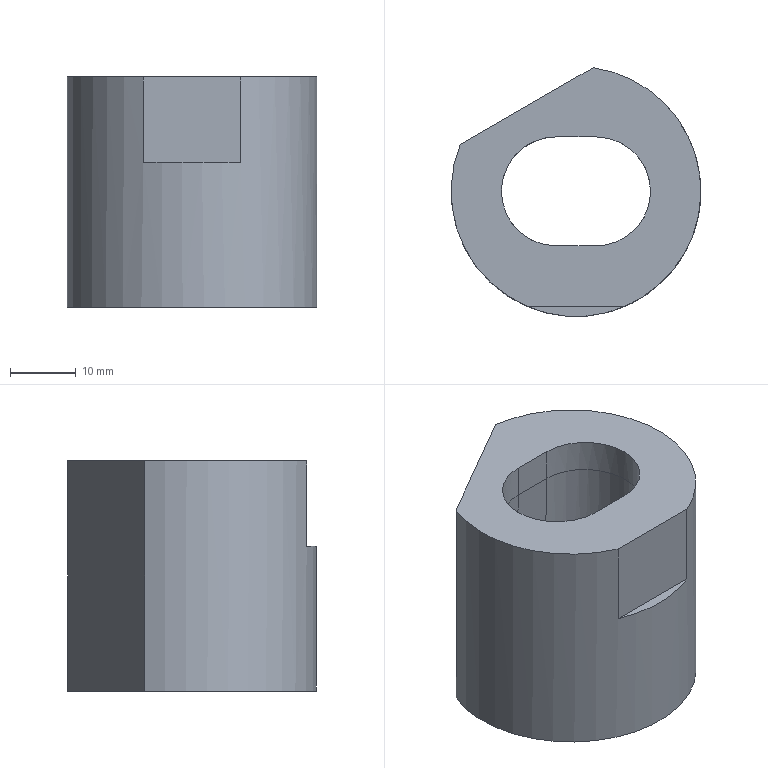Part | STEP file | 1_id4530_x_t | 1 solid | 14 faces | box 38 x 37.821 x 35 mm | volume 25400 mm3 | plane 9 | spline 4 | cylinder 1 | commonest cylinder face diameters 38 x1
STEP:
#1=CARTESIAN_POINT('',(3346.835,-68.341,-35.));
#2=VERTEX_POINT('',#1);
#3=CARTESIAN_POINT('',(3367.034,-56.679,-35.));
#4=VERTEX_POINT('',#3);
#5=CARTESIAN_POINT('',(3354.229,-64.072,-35.));
#6=DIRECTION('',(0.866,0.5,0.));
#7=VECTOR('',#6,1.);
#8=LINE('',#5,#7);
#9=EDGE_CURVE('',#2,#4,#8,.T.);
#10=ORIENTED_EDGE('',*,*,#9,.T.);
#11=CARTESIAN_POINT('',(3364.435,-75.5,-35.));
#12=DIRECTION('',(0.,0.,-1.));
#13=DIRECTION('',(-1.,0.,0.));
#14=AXIS2_PLACEMENT_3D('',#11,#12,#13);
#15=CIRCLE('',#14,19.);
#16=EDGE_CURVE('',#4,#2,#15,.T.);
#17=ORIENTED_EDGE('',*,*,#16,.T.);
#18=EDGE_LOOP('',(#10,#17));
#19=FACE_BOUND('',#18,.T.);
#20=CARTESIAN_POINT('',(3361.37,-84.571,-35.));
#21=VERTEX_POINT('',#20);
#22=CARTESIAN_POINT('',(3361.37,-66.429,-35.));
#23=VERTEX_POINT('',#22);
#24=CARTESIAN_POINT('',(3361.37,-84.571,-35.));
#25=CARTESIAN_POINT('',(3358.983,-84.57,-35.));
#26=CARTESIAN_POINT('',(3356.635,-83.594,-35.));
#27=CARTESIAN_POINT('',(3353.275,-80.233,-35.));
#28=CARTESIAN_POINT('',(3352.301,-77.881,-35.));
#29=CARTESIAN_POINT('',(3352.297,-73.134,-35.));
#30=CARTESIAN_POINT('',(3353.257,-70.789,-35.));
#31=CARTESIAN_POINT('',(3356.642,-67.396,-35.));
#32=CARTESIAN_POINT('',(3358.969,-66.43,-35.));
#33=CARTESIAN_POINT('',(3361.37,-66.429,-35.));
#34=CARTESIAN_POINT('',(3361.37,-66.429,-35.));
#35=CARTESIAN_POINT('',(3361.37,-66.429,-35.));
#36=B_SPLINE_CURVE_WITH_KNOTS('',3,(#24,#25,#26,#27,#28,#29,#30,#31,#32,#33,#34,#35),.UNSPECIFIED.,.F.,.F.,(4,2,2,2,2,4),(0.,0.25,0.5,0.75,1.,1.),.UNSPECIFIED.);
#37=EDGE_CURVE('',#21,#23,#36,.T.);
#38=ORIENTED_EDGE('',*,*,#37,.F.);
#39=CARTESIAN_POINT('',(3367.5,-84.571,-35.));
#40=VERTEX_POINT('',#39);
#41=CARTESIAN_POINT('',(3364.435,-84.571,-35.));
#42=DIRECTION('',(-1.,0.,0.));
#43=VECTOR('',#42,1.);
#44=LINE('',#41,#43);
#45=EDGE_CURVE('',#40,#21,#44,.T.);
#46=ORIENTED_EDGE('',*,*,#45,.F.);
#47=CARTESIAN_POINT('',(3367.5,-66.429,-35.));
#48=VERTEX_POINT('',#47);
#49=CARTESIAN_POINT('',(3367.5,-66.429,-35.));
#50=CARTESIAN_POINT('',(3369.887,-66.43,-35.));
#51=CARTESIAN_POINT('',(3372.235,-67.406,-35.));
#52=CARTESIAN_POINT('',(3375.595,-70.767,-35.));
#53=CARTESIAN_POINT('',(3376.569,-73.119,-35.));
#54=CARTESIAN_POINT('',(3376.573,-77.866,-35.));
#55=CARTESIAN_POINT('',(3375.613,-80.211,-35.));
#56=CARTESIAN_POINT('',(3372.228,-83.604,-35.));
#57=CARTESIAN_POINT('',(3369.901,-84.57,-35.));
#58=CARTESIAN_POINT('',(3367.5,-84.571,-35.));
#59=CARTESIAN_POINT('',(3367.5,-84.571,-35.));
#60=CARTESIAN_POINT('',(3367.5,-84.571,-35.));
#61=B_SPLINE_CURVE_WITH_KNOTS('',3,(#49,#50,#51,#52,#53,#54,#55,#56,#57,#58,#59,#60),.UNSPECIFIED.,.F.,.F.,(4,2,2,2,2,4),(0.,0.25,0.5,0.75,1.,1.),.UNSPECIFIED.);
#62=EDGE_CURVE('',#48,#40,#61,.T.);
#63=ORIENTED_EDGE('',*,*,#62,.F.);
#64=CARTESIAN_POINT('',(3364.435,-66.429,-35.));
#65=DIRECTION('',(1.,0.,0.));
#66=VECTOR('',#65,1.);
#67=LINE('',#64,#66);
#68=EDGE_CURVE('',#23,#48,#67,.T.);
#69=ORIENTED_EDGE('',*,*,#68,.F.);
#70=EDGE_LOOP('',(#38,#46,#63,#69));
#71=FACE_BOUND('',#70,.T.);
#72=CARTESIAN_POINT('',(3364.435,-81.75,-35.));
#73=DIRECTION('',(0.,0.,-1.));
#74=DIRECTION('',(0.,-1.,0.));
#75=AXIS2_PLACEMENT_3D('',#72,#73,#74);
#76=PLANE('',#75);
#77=ADVANCED_FACE('',(#19,#71),#76,.T.);
#78=CARTESIAN_POINT('',(3371.834,-93.,0.00001607));
#79=VERTEX_POINT('',#78);
#80=CARTESIAN_POINT('',(3357.036,-93.,0.00001607));
#81=VERTEX_POINT('',#80);
#82=CARTESIAN_POINT('',(3017.015,-93.,0.00001607));
#83=DIRECTION('',(-1.,0.,0.));
#84=VECTOR('',#83,1.);
#85=LINE('',#82,#84);
#86=EDGE_CURVE('',#79,#81,#85,.T.);
#87=ORIENTED_EDGE('',*,*,#86,.F.);
#88=CARTESIAN_POINT('',(3367.034,-56.679,0.00001607));
#89=VERTEX_POINT('',#88);
#90=CARTESIAN_POINT('',(3364.435,-75.5,0.00001607));
#91=DIRECTION('',(0.,0.,1.));
#92=DIRECTION('',(-1.,0.,0.));
#93=AXIS2_PLACEMENT_3D('',#90,#91,#92);
#94=CIRCLE('',#93,19.);
#95=EDGE_CURVE('',#79,#89,#94,.T.);
#96=ORIENTED_EDGE('',*,*,#95,.T.);
#97=CARTESIAN_POINT('',(3346.835,-68.341,0.00001607));
#98=VERTEX_POINT('',#97);
#99=CARTESIAN_POINT('',(3354.229,-64.072,0.00001607));
#100=DIRECTION('',(-0.866,-0.5,0.));
#101=VECTOR('',#100,1.);
#102=LINE('',#99,#101);
#103=EDGE_CURVE('',#89,#98,#102,.T.);
#104=ORIENTED_EDGE('',*,*,#103,.T.);
#105=CARTESIAN_POINT('',(3364.435,-75.5,0.00001607));
#106=DIRECTION('',(0.,0.,1.));
#107=DIRECTION('',(-1.,0.,0.));
#108=AXIS2_PLACEMENT_3D('',#105,#106,#107);
#109=CIRCLE('',#108,19.);
#110=EDGE_CURVE('',#98,#81,#109,.T.);
#111=ORIENTED_EDGE('',*,*,#110,.T.);
#112=EDGE_LOOP('',(#87,#96,#104,#111));
#113=FACE_BOUND('',#112,.T.);
#114=CARTESIAN_POINT('',(3367.5,-67.215,0.00001607));
#115=VERTEX_POINT('',#114);
#116=CARTESIAN_POINT('',(3367.5,-83.785,0.00001607));
#117=VERTEX_POINT('',#116);
#118=CARTESIAN_POINT('',(3367.5,-67.215,0.00001607));
#119=CARTESIAN_POINT('',(3369.689,-67.215,0.00001607));
#120=CARTESIAN_POINT('',(3371.837,-68.119,0.00001607));
#121=CARTESIAN_POINT('',(3374.884,-71.168,0.00001607));
#122=CARTESIAN_POINT('',(3375.783,-73.333,0.00001607));
#123=CARTESIAN_POINT('',(3375.787,-77.654,0.00001607));
#124=CARTESIAN_POINT('',(3374.906,-79.809,0.00001607));
#125=CARTESIAN_POINT('',(3371.82,-82.899,0.00001607));
#126=CARTESIAN_POINT('',(3369.688,-83.785,0.00001607));
#127=CARTESIAN_POINT('',(3367.5,-83.785,0.00001607));
#128=B_SPLINE_CURVE_WITH_KNOTS('',3,(#118,#119,#120,#121,#122,#123,#124,#125,#126,#127),.UNSPECIFIED.,.F.,.F.,(4,2,2,2,4),(0.,0.25,0.5,0.75,1.),.UNSPECIFIED.);
#129=EDGE_CURVE('',#115,#117,#128,.T.);
#130=ORIENTED_EDGE('',*,*,#129,.T.);
#131=CARTESIAN_POINT('',(3361.37,-83.785,0.00001607));
#132=VERTEX_POINT('',#131);
#133=CARTESIAN_POINT('',(3364.435,-83.785,0.00001607));
#134=DIRECTION('',(-1.,0.,0.));
#135=VECTOR('',#134,1.);
#136=LINE('',#133,#135);
#137=EDGE_CURVE('',#117,#132,#136,.T.);
#138=ORIENTED_EDGE('',*,*,#137,.T.);
#139=CARTESIAN_POINT('',(3361.37,-67.215,0.00001607));
#140=VERTEX_POINT('',#139);
#141=CARTESIAN_POINT('',(3361.37,-83.785,0.00001609));
#142=CARTESIAN_POINT('',(3360.846,-83.785,0.00001609));
#143=CARTESIAN_POINT('',(3360.289,-83.729,0.00001608));
#144=CARTESIAN_POINT('',(3359.228,-83.514,0.00001608));
#145=CARTESIAN_POINT('',(3358.707,-83.354,0.00001607));
#146=CARTESIAN_POINT('',(3357.204,-82.733,0.00001606));
#147=CARTESIAN_POINT('',(3356.28,-82.127,0.00001605));
#148=CARTESIAN_POINT('',(3353.975,-79.822,0.00001604));
#149=CARTESIAN_POINT('',(3353.085,-77.673,0.00001603));
#150=CARTESIAN_POINT('',(3353.085,-73.327,0.00001603));
#151=CARTESIAN_POINT('',(3353.975,-71.178,0.00001604));
#152=CARTESIAN_POINT('',(3357.048,-68.105,0.00001606));
#153=CARTESIAN_POINT('',(3359.207,-67.215,0.00001608));
#154=CARTESIAN_POINT('',(3361.37,-67.215,0.00001609));
#155=B_SPLINE_CURVE_WITH_KNOTS('',3,(#141,#142,#143,#144,#145,#146,#147,#148,#149,#150,#151,#152,#153,#154),.UNSPECIFIED.,.F.,.F.,(4,2,2,2,2,2,4),(0.,0.0625,0.125,0.25,0.5,0.75,1.),.UNSPECIFIED.);
#156=EDGE_CURVE('',#132,#140,#155,.T.);
#157=ORIENTED_EDGE('',*,*,#156,.T.);
#158=CARTESIAN_POINT('',(3364.435,-67.215,0.00001607));
#159=DIRECTION('',(1.,0.,0.));
#160=VECTOR('',#159,1.);
#161=LINE('',#158,#160);
#162=EDGE_CURVE('',#140,#115,#161,.T.);
#163=ORIENTED_EDGE('',*,*,#162,.T.);
#164=EDGE_LOOP('',(#130,#138,#157,#163));
#165=FACE_BOUND('',#164,.T.);
#166=CARTESIAN_POINT('',(3364.435,-81.75,0.00001607));
#167=DIRECTION('',(0.,0.,1.));
#168=DIRECTION('',(0.,1.,0.));
#169=AXIS2_PLACEMENT_3D('',#166,#167,#168);
#170=PLANE('',#169);
#171=ADVANCED_FACE('',(#113,#165),#170,.T.);
#172=ORIENTED_EDGE('',*,*,#95,.F.);
#173=CARTESIAN_POINT('',(3371.834,-93.,-13.));
#174=VERTEX_POINT('',#173);
#175=CARTESIAN_POINT('',(3371.834,-93.,-17.5));
#176=DIRECTION('',(0.,0.,-1.));
#177=VECTOR('',#176,1.);
#178=LINE('',#175,#177);
#179=EDGE_CURVE('',#79,#174,#178,.T.);
#180=ORIENTED_EDGE('',*,*,#179,.T.);
#181=CARTESIAN_POINT('',(3357.036,-93.,-13.));
#182=VERTEX_POINT('',#181);
#183=CARTESIAN_POINT('',(3364.435,-75.5,-13.));
#184=DIRECTION('',(0.,0.,-1.));
#185=DIRECTION('',(0.866,-0.5,0.));
#186=AXIS2_PLACEMENT_3D('',#183,#184,#185);
#187=CIRCLE('',#186,19.);
#188=EDGE_CURVE('',#174,#182,#187,.T.);
#189=ORIENTED_EDGE('',*,*,#188,.T.);
#190=CARTESIAN_POINT('',(3357.036,-93.,-17.5));
#191=DIRECTION('',(0.,0.,1.));
#192=VECTOR('',#191,1.);
#193=LINE('',#190,#192);
#194=EDGE_CURVE('',#182,#81,#193,.T.);
#195=ORIENTED_EDGE('',*,*,#194,.T.);
#196=ORIENTED_EDGE('',*,*,#110,.F.);
#197=CARTESIAN_POINT('',(3346.835,-68.341,-15.));
#198=DIRECTION('',(0.,0.,-1.));
#199=VECTOR('',#198,1.);
#200=LINE('',#197,#199);
#201=EDGE_CURVE('',#98,#2,#200,.T.);
#202=ORIENTED_EDGE('',*,*,#201,.T.);
#203=ORIENTED_EDGE('',*,*,#16,.F.);
#204=CARTESIAN_POINT('',(3367.034,-56.679,-15.));
#205=DIRECTION('',(0.,0.,1.));
#206=VECTOR('',#205,1.);
#207=LINE('',#204,#206);
#208=EDGE_CURVE('',#4,#89,#207,.T.);
#209=ORIENTED_EDGE('',*,*,#208,.T.);
#210=EDGE_LOOP('',(#172,#180,#189,#195,#196,#202,#203,#209));
#211=FACE_OUTER_BOUND('',#210,.T.);
#212=CARTESIAN_POINT('',(3364.435,-75.5,-17.5));
#213=DIRECTION('',(0.,0.,1.));
#214=DIRECTION('',(0.,1.,0.));
#215=AXIS2_PLACEMENT_3D('',#212,#213,#214);
#216=CYLINDRICAL_SURFACE('',#215,19.);
#217=ADVANCED_FACE('',(#211),#216,.T.);
#218=CARTESIAN_POINT('',(3367.5,-83.785,-5.));
#219=VERTEX_POINT('',#218);
#220=CARTESIAN_POINT('',(3361.37,-83.785,-5.));
#221=VERTEX_POINT('',#220);
#222=CARTESIAN_POINT('',(3367.5,-83.785,-5.));
#223=DIRECTION('',(-1.,0.,0.));
#224=VECTOR('',#223,1.);
#225=LINE('',#222,#224);
#226=EDGE_CURVE('',#219,#221,#225,.T.);
#227=ORIENTED_EDGE('',*,*,#226,.T.);
#228=CARTESIAN_POINT('',(3361.37,-83.785,0.00001605));
#229=DIRECTION('',(-0.000000008,0.,1.));
#230=VECTOR('',#229,1.);
#231=LINE('',#228,#230);
#232=EDGE_CURVE('',#221,#132,#231,.T.);
#233=ORIENTED_EDGE('',*,*,#232,.T.);
#234=ORIENTED_EDGE('',*,*,#137,.F.);
#235=CARTESIAN_POINT('',(3367.5,-83.785,0.0000161));
#236=DIRECTION('',(-0.000000008,0.,1.));
#237=VECTOR('',#236,1.);
#238=LINE('',#235,#237);
#239=EDGE_CURVE('',#219,#117,#238,.T.);
#240=ORIENTED_EDGE('',*,*,#239,.F.);
#241=EDGE_LOOP('',(#227,#233,#234,#240));
#242=FACE_OUTER_BOUND('',#241,.T.);
#243=CARTESIAN_POINT('',(3375.435,-83.785,0.00001616));
#244=DIRECTION('',(0.,1.,0.));
#245=DIRECTION('',(-1.,0.,-0.000000008));
#246=AXIS2_PLACEMENT_3D('',#243,#244,#245);
#247=PLANE('',#246);
#248=ADVANCED_FACE('',(#242),#247,.T.);
#249=CARTESIAN_POINT('',(3367.5,-67.215,-5.));
#250=VERTEX_POINT('',#249);
#251=CARTESIAN_POINT('',(3367.51,-67.215,-5.));
#252=VERTEX_POINT('',#251);
#253=CARTESIAN_POINT('',(3367.5,-67.215,-5.));
#254=CARTESIAN_POINT('',(3367.503,-67.215,-5.));
#255=CARTESIAN_POINT('',(3367.506,-67.215,-5.));
#256=CARTESIAN_POINT('',(3367.51,-67.215,-5.));
#257=B_SPLINE_CURVE_WITH_KNOTS('',3,(#253,#254,#255,#256),.UNSPECIFIED.,.F.,.F.,(4,4),(0.,1.),.UNSPECIFIED.);
#258=EDGE_CURVE('',#250,#252,#257,.T.);
#259=ORIENTED_EDGE('',*,*,#258,.T.);
#260=CARTESIAN_POINT('',(3375.785,-75.494,-5.));
#261=VERTEX_POINT('',#260);
#262=CARTESIAN_POINT('',(3367.51,-67.215,-5.));
#263=CARTESIAN_POINT('',(3368.101,-67.216,-5.));
#264=CARTESIAN_POINT('',(3369.043,-67.278,-5.));
#265=CARTESIAN_POINT('',(3370.755,-67.868,-5.));
#266=CARTESIAN_POINT('',(3371.378,-68.149,-5.));
#267=CARTESIAN_POINT('',(3372.327,-68.761,-4.999));
#268=CARTESIAN_POINT('',(3372.675,-69.023,-4.999));
#269=CARTESIAN_POINT('',(3373.201,-69.478,-5.001));
#270=CARTESIAN_POINT('',(3373.4,-69.679,-5.002));
#271=CARTESIAN_POINT('',(3373.695,-69.994,-5.007));
#272=CARTESIAN_POINT('',(3373.749,-70.057,-5.008));
#273=CARTESIAN_POINT('',(3374.011,-70.375,-5.023));
#274=CARTESIAN_POINT('',(3374.169,-70.573,-5.034));
#275=CARTESIAN_POINT('',(3374.607,-71.234,-5.073));
#276=CARTESIAN_POINT('',(3374.749,-71.495,-5.087));
#277=CARTESIAN_POINT('',(3374.93,-71.844,-5.101));
#278=CARTESIAN_POINT('',(3375.032,-72.055,-5.105));
#279=CARTESIAN_POINT('',(3375.229,-72.525,-5.104));
#280=CARTESIAN_POINT('',(3375.324,-72.779,-5.099));
#281=CARTESIAN_POINT('',(3375.452,-73.192,-5.086));
#282=CARTESIAN_POINT('',(3375.493,-73.334,-5.08));
#283=CARTESIAN_POINT('',(3375.568,-73.63,-5.067));
#284=CARTESIAN_POINT('',(3375.617,-73.85,-5.056));
#285=CARTESIAN_POINT('',(3375.783,-74.752,-5.016));
#286=CARTESIAN_POINT('',(3375.785,-75.246,-5.));
#287=CARTESIAN_POINT('',(3375.785,-75.494,-5.));
#288=B_SPLINE_CURVE_WITH_KNOTS('',3,(#262,#263,#264,#265,#266,#267,#268,#269,#270,#271,#272,#273,#274,#275,#276,#277,#278,#279,#280,#281,#282,#283,#284,#285,#286,#287),.UNSPECIFIED.,.F.,.F.,(4,2,2,2,2,2,2,2,2,2,2,2,4),(0.,0.25,0.375,0.4375,0.5,0.5625,0.625,0.6875,0.75,0.8125,0.8437,0.875,1.),.UNSPECIFIED.);
#289=EDGE_CURVE('',#252,#261,#288,.T.);
#290=ORIENTED_EDGE('',*,*,#289,.T.);
#291=CARTESIAN_POINT('',(3375.444,-77.83,-5.));
#292=VERTEX_POINT('',#291);
#293=CARTESIAN_POINT('',(3375.785,-75.494,-5.));
#294=CARTESIAN_POINT('',(3375.785,-75.496,-5.));
#295=CARTESIAN_POINT('',(3375.785,-75.498,-5.));
#296=CARTESIAN_POINT('',(3375.785,-76.289,-5.));
#297=CARTESIAN_POINT('',(3375.668,-77.076,-5.));
#298=CARTESIAN_POINT('',(3375.444,-77.831,-5.));
#299=B_SPLINE_CURVE_WITH_KNOTS('',3,(#293,#294,#295,#296,#297,#298),.UNSPECIFIED.,.F.,.F.,(4,2,4),(0.,0.002604,1.),.UNSPECIFIED.);
#300=EDGE_CURVE('',#261,#292,#299,.T.);
#301=ORIENTED_EDGE('',*,*,#300,.T.);
#302=CARTESIAN_POINT('',(3373.365,-81.352,-5.));
#303=VERTEX_POINT('',#302);
#304=CARTESIAN_POINT('',(3375.444,-77.831,-5.));
#305=CARTESIAN_POINT('',(3375.054,-79.151,-5.));
#306=CARTESIAN_POINT('',(3374.34,-80.375,-5.));
#307=CARTESIAN_POINT('',(3373.365,-81.352,-5.));
#308=B_SPLINE_CURVE_WITH_KNOTS('',3,(#304,#305,#306,#307),.UNSPECIFIED.,.F.,.F.,(4,4),(0.,1.),.UNSPECIFIED.);
#309=EDGE_CURVE('',#292,#303,#308,.T.);
#310=ORIENTED_EDGE('',*,*,#309,.T.);
#311=CARTESIAN_POINT('',(3367.509,-83.785,-5.));
#312=VERTEX_POINT('',#311);
#313=CARTESIAN_POINT('',(3373.365,-81.352,-5.));
#314=CARTESIAN_POINT('',(3373.363,-81.354,-5.));
#315=CARTESIAN_POINT('',(3373.361,-81.356,-5.));
#316=CARTESIAN_POINT('',(3372.59,-82.127,-5.));
#317=CARTESIAN_POINT('',(3371.666,-82.733,-5.));
#318=CARTESIAN_POINT('',(3370.163,-83.354,-5.));
#319=CARTESIAN_POINT('',(3369.642,-83.514,-5.));
#320=CARTESIAN_POINT('',(3368.584,-83.728,-5.));
#321=CARTESIAN_POINT('',(3368.03,-83.784,-5.));
#322=CARTESIAN_POINT('',(3367.509,-83.785,-5.));
#323=B_SPLINE_CURVE_WITH_KNOTS('',3,(#313,#314,#315,#316,#317,#318,#319,#320,#321,#322),.UNSPECIFIED.,.F.,.F.,(4,2,2,2,4),(0.,0.001413,0.5014,0.7514,1.),.UNSPECIFIED.);
#324=EDGE_CURVE('',#303,#312,#323,.T.);
#325=ORIENTED_EDGE('',*,*,#324,.T.);
#326=CARTESIAN_POINT('',(3367.509,-83.785,-5.));
#327=CARTESIAN_POINT('',(3367.506,-83.785,-5.));
#328=CARTESIAN_POINT('',(3367.503,-83.785,-5.));
#329=CARTESIAN_POINT('',(3367.5,-83.785,-5.));
#330=B_SPLINE_CURVE_WITH_KNOTS('',3,(#326,#327,#328,#329),.UNSPECIFIED.,.F.,.F.,(4,4),(0.,1.),.UNSPECIFIED.);
#331=EDGE_CURVE('',#312,#219,#330,.T.);
#332=ORIENTED_EDGE('',*,*,#331,.T.);
#333=ORIENTED_EDGE('',*,*,#239,.T.);
#334=ORIENTED_EDGE('',*,*,#129,.F.);
#335=CARTESIAN_POINT('',(3367.5,-67.215,0.0000161));
#336=DIRECTION('',(-0.000000008,0.,1.));
#337=VECTOR('',#336,1.);
#338=LINE('',#335,#337);
#339=EDGE_CURVE('',#250,#115,#338,.T.);
#340=ORIENTED_EDGE('',*,*,#339,.F.);
#341=EDGE_LOOP('',(#259,#290,#301,#310,#325,#332,#333,#334,#340));
#342=FACE_OUTER_BOUND('',#341,.T.);
#343=CARTESIAN_POINT('',(3367.5,-67.215,-5.146));
#344=CARTESIAN_POINT('',(3367.5,-67.215,0.00001607));
#345=CARTESIAN_POINT('',(3368.024,-67.215,-5.146));
#346=CARTESIAN_POINT('',(3368.024,-67.215,0.00001608));
#347=CARTESIAN_POINT('',(3368.581,-67.271,-5.146));
#348=CARTESIAN_POINT('',(3368.581,-67.271,0.00001608));
#349=CARTESIAN_POINT('',(3369.642,-67.486,-5.146));
#350=CARTESIAN_POINT('',(3369.642,-67.486,0.00001609));
#351=CARTESIAN_POINT('',(3370.163,-67.646,-5.146));
#352=CARTESIAN_POINT('',(3370.163,-67.646,0.00001609));
#353=CARTESIAN_POINT('',(3371.666,-68.267,-5.146));
#354=CARTESIAN_POINT('',(3371.666,-68.267,0.00001611));
#355=CARTESIAN_POINT('',(3372.59,-68.873,-5.146));
#356=CARTESIAN_POINT('',(3372.59,-68.873,0.00001611));
#357=CARTESIAN_POINT('',(3374.895,-71.178,-5.146));
#358=CARTESIAN_POINT('',(3374.895,-71.178,0.00001613));
#359=CARTESIAN_POINT('',(3375.785,-73.327,-5.146));
#360=CARTESIAN_POINT('',(3375.785,-73.327,0.00001614));
#361=CARTESIAN_POINT('',(3375.785,-77.673,-5.146));
#362=CARTESIAN_POINT('',(3375.785,-77.673,0.00001614));
#363=CARTESIAN_POINT('',(3374.895,-79.822,-5.146));
#364=CARTESIAN_POINT('',(3374.895,-79.822,0.00001613));
#365=CARTESIAN_POINT('',(3372.59,-82.127,-5.146));
#366=CARTESIAN_POINT('',(3372.59,-82.127,0.00001611));
#367=CARTESIAN_POINT('',(3371.666,-82.733,-5.146));
#368=CARTESIAN_POINT('',(3371.666,-82.733,0.00001611));
#369=CARTESIAN_POINT('',(3370.163,-83.354,-5.146));
#370=CARTESIAN_POINT('',(3370.163,-83.354,0.00001609));
#371=CARTESIAN_POINT('',(3369.642,-83.514,-5.146));
#372=CARTESIAN_POINT('',(3369.642,-83.514,0.00001609));
#373=CARTESIAN_POINT('',(3368.581,-83.729,-5.146));
#374=CARTESIAN_POINT('',(3368.581,-83.729,0.00001608));
#375=CARTESIAN_POINT('',(3368.024,-83.785,-5.146));
#376=CARTESIAN_POINT('',(3368.024,-83.785,0.00001608));
#377=CARTESIAN_POINT('',(3367.5,-83.785,-5.146));
#378=CARTESIAN_POINT('',(3367.5,-83.785,0.00001607));
#379=B_SPLINE_SURFACE_WITH_KNOTS('',3,1,((#343,#344),(#345,#346),(#347,#348),(#349,#350),(#351,#352),(#353,#354),(#355,#356),(#357,#358),(#359,#360),(#361,#362),(#363,#364),(#365,#366),(#367,#368),(#369,#370),(#371,#372),(#373,#374),(#375,#376),(#377,#378)),.UNSPECIFIED.,.F.,.F.,.F.,(4,2,2,2,2,2,2,2,4),(2,2),(0.,0.0625,0.125,0.25,0.5,0.75,0.875,0.9375,1.),(0.,1.),.UNSPECIFIED.);
#380=ADVANCED_FACE('',(#342),#379,.T.);
#381=CARTESIAN_POINT('',(3361.37,-67.215,-5.));
#382=VERTEX_POINT('',#381);
#383=CARTESIAN_POINT('',(3361.37,-67.215,-5.));
#384=DIRECTION('',(1.,0.,0.));
#385=VECTOR('',#384,1.);
#386=LINE('',#383,#385);
#387=EDGE_CURVE('',#382,#250,#386,.T.);
#388=ORIENTED_EDGE('',*,*,#387,.T.);
#389=ORIENTED_EDGE('',*,*,#339,.T.);
#390=ORIENTED_EDGE('',*,*,#162,.F.);
#391=CARTESIAN_POINT('',(3361.37,-67.215,0.00001605));
#392=DIRECTION('',(-0.000000008,0.,1.));
#393=VECTOR('',#392,1.);
#394=LINE('',#391,#393);
#395=EDGE_CURVE('',#382,#140,#394,.T.);
#396=ORIENTED_EDGE('',*,*,#395,.F.);
#397=EDGE_LOOP('',(#388,#389,#390,#396));
#398=FACE_OUTER_BOUND('',#397,.T.);
#399=CARTESIAN_POINT('',(3375.435,-67.215,0.00001616));
#400=DIRECTION('',(0.,-1.,0.));
#401=DIRECTION('',(1.,0.,0.000000008));
#402=AXIS2_PLACEMENT_3D('',#399,#400,#401);
#403=PLANE('',#402);
#404=ADVANCED_FACE('',(#398),#403,.T.);
#405=CARTESIAN_POINT('',(3361.36,-83.785,-5.));
#406=VERTEX_POINT('',#405);
#407=CARTESIAN_POINT('',(3361.37,-83.785,-5.));
#408=CARTESIAN_POINT('',(3361.367,-83.785,-5.));
#409=CARTESIAN_POINT('',(3361.364,-83.785,-5.));
#410=CARTESIAN_POINT('',(3361.36,-83.785,-5.));
#411=B_SPLINE_CURVE_WITH_KNOTS('',3,(#407,#408,#409,#410),.UNSPECIFIED.,.F.,.F.,(4,4),(0.,1.),.UNSPECIFIED.);
#412=EDGE_CURVE('',#221,#406,#411,.T.);
#413=ORIENTED_EDGE('',*,*,#412,.T.);
#414=CARTESIAN_POINT('',(3353.085,-75.506,-5.));
#415=VERTEX_POINT('',#414);
#416=CARTESIAN_POINT('',(3361.36,-83.785,-5.));
#417=CARTESIAN_POINT('',(3360.769,-83.784,-5.));
#418=CARTESIAN_POINT('',(3359.827,-83.722,-5.));
#419=CARTESIAN_POINT('',(3358.115,-83.132,-5.));
#420=CARTESIAN_POINT('',(3357.492,-82.851,-5.));
#421=CARTESIAN_POINT('',(3356.543,-82.239,-4.999));
#422=CARTESIAN_POINT('',(3356.195,-81.977,-4.999));
#423=CARTESIAN_POINT('',(3355.669,-81.522,-5.001));
#424=CARTESIAN_POINT('',(3355.47,-81.321,-5.002));
#425=CARTESIAN_POINT('',(3355.175,-81.006,-5.007));
#426=CARTESIAN_POINT('',(3355.121,-80.943,-5.008));
#427=CARTESIAN_POINT('',(3354.859,-80.625,-5.023));
#428=CARTESIAN_POINT('',(3354.701,-80.427,-5.034));
#429=CARTESIAN_POINT('',(3354.263,-79.766,-5.073));
#430=CARTESIAN_POINT('',(3354.121,-79.505,-5.087));
#431=CARTESIAN_POINT('',(3353.94,-79.156,-5.101));
#432=CARTESIAN_POINT('',(3353.838,-78.945,-5.105));
#433=CARTESIAN_POINT('',(3353.641,-78.475,-5.104));
#434=CARTESIAN_POINT('',(3353.546,-78.221,-5.099));
#435=CARTESIAN_POINT('',(3353.418,-77.808,-5.086));
#436=CARTESIAN_POINT('',(3353.377,-77.666,-5.08));
#437=CARTESIAN_POINT('',(3353.302,-77.37,-5.067));
#438=CARTESIAN_POINT('',(3353.253,-77.15,-5.056));
#439=CARTESIAN_POINT('',(3353.087,-76.248,-5.016));
#440=CARTESIAN_POINT('',(3353.085,-75.754,-5.));
#441=CARTESIAN_POINT('',(3353.085,-75.506,-5.));
#442=B_SPLINE_CURVE_WITH_KNOTS('',3,(#416,#417,#418,#419,#420,#421,#422,#423,#424,#425,#426,#427,#428,#429,#430,#431,#432,#433,#434,#435,#436,#437,#438,#439,#440,#441),.UNSPECIFIED.,.F.,.F.,(4,2,2,2,2,2,2,2,2,2,2,2,4),(0.,0.25,0.375,0.4375,0.5,0.5625,0.625,0.6875,0.75,0.8125,0.8437,0.875,1.),.UNSPECIFIED.);
#443=EDGE_CURVE('',#406,#415,#442,.T.);
#444=ORIENTED_EDGE('',*,*,#443,.T.);
#445=CARTESIAN_POINT('',(3353.426,-73.17,-5.));
#446=VERTEX_POINT('',#445);
#447=CARTESIAN_POINT('',(3353.085,-75.506,-5.));
#448=CARTESIAN_POINT('',(3353.085,-75.504,-5.));
#449=CARTESIAN_POINT('',(3353.085,-75.502,-5.));
#450=CARTESIAN_POINT('',(3353.085,-74.711,-5.));
#451=CARTESIAN_POINT('',(3353.202,-73.925,-5.));
#452=CARTESIAN_POINT('',(3353.425,-73.17,-5.));
#453=B_SPLINE_CURVE_WITH_KNOTS('',3,(#447,#448,#449,#450,#451,#452),.UNSPECIFIED.,.F.,.F.,(4,2,4),(0.,0.002605,1.),.UNSPECIFIED.);
#454=EDGE_CURVE('',#415,#446,#453,.T.);
#455=ORIENTED_EDGE('',*,*,#454,.T.);
#456=CARTESIAN_POINT('',(3355.505,-69.648,-5.));
#457=VERTEX_POINT('',#456);
#458=CARTESIAN_POINT('',(3353.425,-73.17,-5.));
#459=CARTESIAN_POINT('',(3353.816,-71.85,-5.));
#460=CARTESIAN_POINT('',(3354.53,-70.625,-5.));
#461=CARTESIAN_POINT('',(3355.505,-69.648,-5.));
#462=B_SPLINE_CURVE_WITH_KNOTS('',3,(#458,#459,#460,#461),.UNSPECIFIED.,.F.,.F.,(4,4),(0.,1.),.UNSPECIFIED.);
#463=EDGE_CURVE('',#446,#457,#462,.T.);
#464=ORIENTED_EDGE('',*,*,#463,.T.);
#465=CARTESIAN_POINT('',(3361.361,-67.215,-5.));
#466=VERTEX_POINT('',#465);
#467=CARTESIAN_POINT('',(3355.505,-69.648,-5.));
#468=CARTESIAN_POINT('',(3355.507,-69.646,-5.));
#469=CARTESIAN_POINT('',(3355.509,-69.644,-5.));
#470=CARTESIAN_POINT('',(3357.046,-68.107,-5.));
#471=CARTESIAN_POINT('',(3359.201,-67.218,-5.));
#472=CARTESIAN_POINT('',(3361.361,-67.215,-5.));
#473=B_SPLINE_CURVE_WITH_KNOTS('',3,(#467,#468,#469,#470,#471,#472),.UNSPECIFIED.,.F.,.F.,(4,2,4),(0.,0.00141,1.),.UNSPECIFIED.);
#474=EDGE_CURVE('',#457,#466,#473,.T.);
#475=ORIENTED_EDGE('',*,*,#474,.T.);
#476=CARTESIAN_POINT('',(3361.361,-67.215,-5.));
#477=CARTESIAN_POINT('',(3361.364,-67.215,-5.));
#478=CARTESIAN_POINT('',(3361.367,-67.215,-5.));
#479=CARTESIAN_POINT('',(3361.37,-67.215,-5.));
#480=B_SPLINE_CURVE_WITH_KNOTS('',3,(#476,#477,#478,#479),.UNSPECIFIED.,.F.,.F.,(4,4),(0.,1.),.UNSPECIFIED.);
#481=EDGE_CURVE('',#466,#382,#480,.T.);
#482=ORIENTED_EDGE('',*,*,#481,.T.);
#483=ORIENTED_EDGE('',*,*,#395,.T.);
#484=ORIENTED_EDGE('',*,*,#156,.F.);
#485=ORIENTED_EDGE('',*,*,#232,.F.);
#486=EDGE_LOOP('',(#413,#444,#455,#464,#475,#482,#483,#484,#485));
#487=FACE_OUTER_BOUND('',#486,.T.);
#488=CARTESIAN_POINT('',(3361.37,-83.785,-5.146));
#489=CARTESIAN_POINT('',(3361.37,-83.785,0.00001611));
#490=CARTESIAN_POINT('',(3360.846,-83.785,-5.146));
#491=CARTESIAN_POINT('',(3360.846,-83.785,0.0000161));
#492=CARTESIAN_POINT('',(3360.289,-83.729,-5.146));
#493=CARTESIAN_POINT('',(3360.289,-83.729,0.0000161));
#494=CARTESIAN_POINT('',(3359.228,-83.514,-5.146));
#495=CARTESIAN_POINT('',(3359.228,-83.514,0.00001609));
#496=CARTESIAN_POINT('',(3358.707,-83.354,-5.146));
#497=CARTESIAN_POINT('',(3358.707,-83.354,0.00001608));
#498=CARTESIAN_POINT('',(3357.204,-82.733,-5.146));
#499=CARTESIAN_POINT('',(3357.204,-82.733,0.00001607));
#500=CARTESIAN_POINT('',(3356.28,-82.127,-5.146));
#501=CARTESIAN_POINT('',(3356.28,-82.127,0.00001607));
#502=CARTESIAN_POINT('',(3353.975,-79.822,-5.146));
#503=CARTESIAN_POINT('',(3353.975,-79.822,0.00001605));
#504=CARTESIAN_POINT('',(3353.085,-77.673,-5.146));
#505=CARTESIAN_POINT('',(3353.085,-77.673,0.00001604));
#506=CARTESIAN_POINT('',(3353.085,-73.327,-5.146));
#507=CARTESIAN_POINT('',(3353.085,-73.327,0.00001604));
#508=CARTESIAN_POINT('',(3353.975,-71.178,-5.146));
#509=CARTESIAN_POINT('',(3353.975,-71.178,0.00001605));
#510=CARTESIAN_POINT('',(3357.048,-68.105,-5.146));
#511=CARTESIAN_POINT('',(3357.048,-68.105,0.00001607));
#512=CARTESIAN_POINT('',(3359.207,-67.215,-5.146));
#513=CARTESIAN_POINT('',(3359.207,-67.215,0.00001609));
#514=CARTESIAN_POINT('',(3361.37,-67.215,-5.146));
#515=CARTESIAN_POINT('',(3361.37,-67.215,0.00001611));
#516=B_SPLINE_SURFACE_WITH_KNOTS('',3,1,((#488,#489),(#490,#491),(#492,#493),(#494,#495),(#496,#497),(#498,#499),(#500,#501),(#502,#503),(#504,#505),(#506,#507),(#508,#509),(#510,#511),(#512,#513),(#514,#515)),.UNSPECIFIED.,.F.,.F.,.F.,(4,2,2,2,2,2,4),(2,2),(0.,0.0625,0.125,0.25,0.5,0.75,1.),(0.,1.),.UNSPECIFIED.);
#517=ADVANCED_FACE('',(#487),#516,.T.);
#518=ORIENTED_EDGE('',*,*,#9,.F.);
#519=ORIENTED_EDGE('',*,*,#201,.F.);
#520=ORIENTED_EDGE('',*,*,#103,.F.);
#521=ORIENTED_EDGE('',*,*,#208,.F.);
#522=EDGE_LOOP('',(#518,#519,#520,#521));
#523=FACE_OUTER_BOUND('',#522,.T.);
#524=CARTESIAN_POINT('',(3356.935,-62.51,-32.5));
#525=DIRECTION('',(-0.5,0.866,0.));
#526=DIRECTION('',(-0.866,-0.5,0.));
#527=AXIS2_PLACEMENT_3D('',#524,#525,#526);
#528=PLANE('',#527);
#529=ADVANCED_FACE('',(#523),#528,.T.);
#530=ORIENTED_EDGE('',*,*,#62,.T.);
#531=CARTESIAN_POINT('',(3367.5,-83.785,-5.));
#532=DIRECTION('',(0.,-0.02618,-0.9997));
#533=VECTOR('',#532,1.);
#534=LINE('',#531,#533);
#535=EDGE_CURVE('',#219,#40,#534,.T.);
#536=ORIENTED_EDGE('',*,*,#535,.F.);
#537=ORIENTED_EDGE('',*,*,#331,.F.);
#538=ORIENTED_EDGE('',*,*,#324,.F.);
#539=ORIENTED_EDGE('',*,*,#309,.F.);
#540=ORIENTED_EDGE('',*,*,#300,.F.);
#541=ORIENTED_EDGE('',*,*,#289,.F.);
#542=ORIENTED_EDGE('',*,*,#258,.F.);
#543=CARTESIAN_POINT('',(3367.5,-67.215,-5.));
#544=DIRECTION('',(0.000004048,0.02618,-0.9997));
#545=VECTOR('',#544,1.);
#546=LINE('',#543,#545);
#547=EDGE_CURVE('',#250,#48,#546,.T.);
#548=ORIENTED_EDGE('',*,*,#547,.T.);
#549=EDGE_LOOP('',(#530,#536,#537,#538,#539,#540,#541,#542,#548));
#550=FACE_OUTER_BOUND('',#549,.T.);
#551=CARTESIAN_POINT('',(3367.5,-67.226,-4.58));
#552=CARTESIAN_POINT('',(3369.667,-67.226,-4.58));
#553=CARTESIAN_POINT('',(3371.827,-68.125,-4.58));
#554=CARTESIAN_POINT('',(3374.876,-71.175,-4.58));
#555=CARTESIAN_POINT('',(3375.772,-73.339,-4.58));
#556=CARTESIAN_POINT('',(3375.776,-77.646,-4.58));
#557=CARTESIAN_POINT('',(3374.897,-79.801,-4.58));
#558=CARTESIAN_POINT('',(3371.816,-82.888,-4.58));
#559=CARTESIAN_POINT('',(3369.686,-83.774,-4.58));
#560=CARTESIAN_POINT('',(3367.413,-83.774,-4.58));
#561=CARTESIAN_POINT('',(3367.325,-83.774,-4.58));
#562=CARTESIAN_POINT('',(3367.238,-83.774,-4.58));
#563=CARTESIAN_POINT('',(3367.5,-67.215,-5.));
#564=CARTESIAN_POINT('',(3369.67,-67.215,-5.));
#565=CARTESIAN_POINT('',(3371.833,-68.115,-5.));
#566=CARTESIAN_POINT('',(3374.886,-71.169,-5.));
#567=CARTESIAN_POINT('',(3375.783,-73.336,-5.));
#568=CARTESIAN_POINT('',(3375.787,-77.649,-5.));
#569=CARTESIAN_POINT('',(3374.907,-79.807,-5.));
#570=CARTESIAN_POINT('',(3371.822,-82.898,-5.));
#571=CARTESIAN_POINT('',(3369.689,-83.785,-5.));
#572=CARTESIAN_POINT('',(3367.412,-83.785,-5.));
#573=CARTESIAN_POINT('',(3367.325,-83.785,-5.));
#574=CARTESIAN_POINT('',(3367.237,-83.785,-5.));
#575=CARTESIAN_POINT('',(3367.5,-66.115,-47.));
#576=CARTESIAN_POINT('',(3369.973,-66.116,-47.));
#577=CARTESIAN_POINT('',(3372.395,-67.123,-47.));
#578=CARTESIAN_POINT('',(3375.878,-70.607,-47.));
#579=CARTESIAN_POINT('',(3376.883,-73.032,-47.));
#580=CARTESIAN_POINT('',(3376.887,-77.952,-47.));
#581=CARTESIAN_POINT('',(3375.896,-80.373,-47.));
#582=CARTESIAN_POINT('',(3372.39,-83.886,-47.));
#583=CARTESIAN_POINT('',(3369.985,-84.884,-47.));
#584=CARTESIAN_POINT('',(3367.401,-84.885,-47.));
#585=CARTESIAN_POINT('',(3367.301,-84.885,-47.));
#586=CARTESIAN_POINT('',(3367.202,-84.885,-47.));
#587=B_SPLINE_SURFACE_WITH_KNOTS('',1,3,((#551,#552,#553,#554,#555,#556,#557,#558,#559,#560,#561,#562),(#563,#564,#565,#566,#567,#568,#569,#570,#571,#572,#573,#574),(#575,#576,#577,#578,#579,#580,#581,#582,#583,#584,#585,#586)),.UNSPECIFIED.,.F.,.F.,.F.,(2,1,2),(4,2,2,2,2,4),(0.,0.009901,1.),(0.,0.2475,0.495,0.7426,0.9901,1.),.UNSPECIFIED.);
#588=ADVANCED_FACE('',(#550),#587,.T.);
#589=ORIENTED_EDGE('',*,*,#68,.T.);
#590=ORIENTED_EDGE('',*,*,#547,.F.);
#591=ORIENTED_EDGE('',*,*,#387,.F.);
#592=CARTESIAN_POINT('',(3361.37,-67.215,-5.));
#593=DIRECTION('',(0.,0.02618,-0.9997));
#594=VECTOR('',#593,1.);
#595=LINE('',#592,#594);
#596=EDGE_CURVE('',#382,#23,#595,.T.);
#597=ORIENTED_EDGE('',*,*,#596,.T.);
#598=EDGE_LOOP('',(#589,#590,#591,#597));
#599=FACE_OUTER_BOUND('',#598,.T.);
#600=CARTESIAN_POINT('',(3361.37,-67.215,-5.));
#601=DIRECTION('',(0.,-0.9997,-0.02618));
#602=DIRECTION('',(0.,0.02618,-0.9997));
#603=AXIS2_PLACEMENT_3D('',#600,#601,#602);
#604=PLANE('',#603);
#605=ADVANCED_FACE('',(#599),#604,.T.);
#606=ORIENTED_EDGE('',*,*,#37,.T.);
#607=ORIENTED_EDGE('',*,*,#596,.F.);
#608=ORIENTED_EDGE('',*,*,#481,.F.);
#609=ORIENTED_EDGE('',*,*,#474,.F.);
#610=ORIENTED_EDGE('',*,*,#463,.F.);
#611=ORIENTED_EDGE('',*,*,#454,.F.);
#612=ORIENTED_EDGE('',*,*,#443,.F.);
#613=ORIENTED_EDGE('',*,*,#412,.F.);
#614=CARTESIAN_POINT('',(3361.37,-83.785,-5.));
#615=DIRECTION('',(-0.000004048,-0.02618,-0.9997));
#616=VECTOR('',#615,1.);
#617=LINE('',#614,#616);
#618=EDGE_CURVE('',#221,#21,#617,.T.);
#619=ORIENTED_EDGE('',*,*,#618,.T.);
#620=EDGE_LOOP('',(#606,#607,#608,#609,#610,#611,#612,#613,#619));
#621=FACE_OUTER_BOUND('',#620,.T.);
#622=CARTESIAN_POINT('',(3361.37,-83.774,-4.58));
#623=CARTESIAN_POINT('',(3359.203,-83.774,-4.58));
#624=CARTESIAN_POINT('',(3357.043,-82.875,-4.58));
#625=CARTESIAN_POINT('',(3353.994,-79.825,-4.58));
#626=CARTESIAN_POINT('',(3353.098,-77.661,-4.58));
#627=CARTESIAN_POINT('',(3353.094,-73.354,-4.58));
#628=CARTESIAN_POINT('',(3353.973,-71.199,-4.58));
#629=CARTESIAN_POINT('',(3357.054,-68.112,-4.58));
#630=CARTESIAN_POINT('',(3359.184,-67.226,-4.58));
#631=CARTESIAN_POINT('',(3361.457,-67.226,-4.58));
#632=CARTESIAN_POINT('',(3361.545,-67.226,-4.58));
#633=CARTESIAN_POINT('',(3361.632,-67.226,-4.58));
#634=CARTESIAN_POINT('',(3361.37,-83.785,-5.));
#635=CARTESIAN_POINT('',(3359.2,-83.785,-5.));
#636=CARTESIAN_POINT('',(3357.037,-82.885,-5.));
#637=CARTESIAN_POINT('',(3353.984,-79.831,-5.));
#638=CARTESIAN_POINT('',(3353.087,-77.664,-5.));
#639=CARTESIAN_POINT('',(3353.083,-73.351,-5.));
#640=CARTESIAN_POINT('',(3353.963,-71.193,-5.));
#641=CARTESIAN_POINT('',(3357.048,-68.102,-5.));
#642=CARTESIAN_POINT('',(3359.181,-67.215,-5.));
#643=CARTESIAN_POINT('',(3361.457,-67.215,-5.));
#644=CARTESIAN_POINT('',(3361.545,-67.215,-5.));
#645=CARTESIAN_POINT('',(3361.633,-67.215,-5.));
#646=CARTESIAN_POINT('',(3361.37,-84.885,-47.));
#647=CARTESIAN_POINT('',(3358.897,-84.884,-47.));
#648=CARTESIAN_POINT('',(3356.475,-83.877,-47.));
#649=CARTESIAN_POINT('',(3352.992,-80.393,-47.));
#650=CARTESIAN_POINT('',(3351.987,-77.968,-47.));
#651=CARTESIAN_POINT('',(3351.983,-73.048,-47.));
#652=CARTESIAN_POINT('',(3352.974,-70.627,-47.));
#653=CARTESIAN_POINT('',(3356.48,-67.114,-47.));
#654=CARTESIAN_POINT('',(3358.885,-66.116,-47.));
#655=CARTESIAN_POINT('',(3361.469,-66.115,-47.));
#656=CARTESIAN_POINT('',(3361.569,-66.115,-47.));
#657=CARTESIAN_POINT('',(3361.668,-66.115,-47.));
#658=B_SPLINE_SURFACE_WITH_KNOTS('',1,3,((#622,#623,#624,#625,#626,#627,#628,#629,#630,#631,#632,#633),(#634,#635,#636,#637,#638,#639,#640,#641,#642,#643,#644,#645),(#646,#647,#648,#649,#650,#651,#652,#653,#654,#655,#656,#657)),.UNSPECIFIED.,.F.,.F.,.F.,(2,1,2),(4,2,2,2,2,4),(0.,0.009901,1.),(0.,0.2475,0.495,0.7426,0.9901,1.),.UNSPECIFIED.);
#659=ADVANCED_FACE('',(#621),#658,.T.);
#660=ORIENTED_EDGE('',*,*,#45,.T.);
#661=ORIENTED_EDGE('',*,*,#618,.F.);
#662=ORIENTED_EDGE('',*,*,#226,.F.);
#663=ORIENTED_EDGE('',*,*,#535,.T.);
#664=EDGE_LOOP('',(#660,#661,#662,#663));
#665=FACE_OUTER_BOUND('',#664,.T.);
#666=CARTESIAN_POINT('',(3367.5,-83.785,-5.));
#667=DIRECTION('',(0.,0.9997,-0.02618));
#668=DIRECTION('',(0.,0.02618,0.9997));
#669=AXIS2_PLACEMENT_3D('',#666,#667,#668);
#670=PLANE('',#669);
#671=ADVANCED_FACE('',(#665),#670,.T.);
#672=ORIENTED_EDGE('',*,*,#179,.F.);
#673=ORIENTED_EDGE('',*,*,#86,.T.);
#674=ORIENTED_EDGE('',*,*,#194,.F.);
#675=CARTESIAN_POINT('',(3017.015,-93.,-13.));
#676=DIRECTION('',(1.,0.,0.));
#677=VECTOR('',#676,1.);
#678=LINE('',#675,#677);
#679=EDGE_CURVE('',#182,#174,#678,.T.);
#680=ORIENTED_EDGE('',*,*,#679,.T.);
#681=EDGE_LOOP('',(#672,#673,#674,#680));
#682=FACE_OUTER_BOUND('',#681,.T.);
#683=CARTESIAN_POINT('',(3017.015,-93.,0.));
#684=DIRECTION('',(0.,-1.,0.));
#685=DIRECTION('',(0.,0.,1.));
#686=AXIS2_PLACEMENT_3D('',#683,#684,#685);
#687=PLANE('',#686);
#688=ADVANCED_FACE('',(#682),#687,.T.);
#689=ORIENTED_EDGE('',*,*,#679,.F.);
#690=ORIENTED_EDGE('',*,*,#188,.F.);
#691=EDGE_LOOP('',(#689,#690));
#692=FACE_OUTER_BOUND('',#691,.T.);
#693=CARTESIAN_POINT('',(3356.435,-101.,-13.));
#694=DIRECTION('',(0.,0.,1.));
#695=DIRECTION('',(0.,1.,0.));
#696=AXIS2_PLACEMENT_3D('',#693,#694,#695);
#697=PLANE('',#696);
#698=ADVANCED_FACE('',(#692),#697,.T.);
#699=CLOSED_SHELL('',(#77,#171,#217,#248,#380,#404,#517,#529,#588,#605,#659,#671,#688,#698));
#700=MANIFOLD_SOLID_BREP('',#699);
#701=(LENGTH_UNIT()NAMED_UNIT(*)SI_UNIT(.MILLI.,.METRE.));
#702=UNCERTAINTY_MEASURE_WITH_UNIT(LENGTH_MEASURE(0.0508),#701,'','');
#703=(NAMED_UNIT(*)PLANE_ANGLE_UNIT()SI_UNIT($,.RADIAN.));
#704=PLANE_ANGLE_MEASURE_WITH_UNIT(PLANE_ANGLE_MEASURE(0.01745),#703);
#705=DIMENSIONAL_EXPONENTS(0.,0.,0.,0.,0.,0.,0.);
#706=(CONVERSION_BASED_UNIT('DEGREE',#704)NAMED_UNIT(#705)PLANE_ANGLE_UNIT());
#707=(NAMED_UNIT(*)SI_UNIT($,.STERADIAN.)SOLID_ANGLE_UNIT());
#708=(GEOMETRIC_REPRESENTATION_CONTEXT(3)GLOBAL_UNCERTAINTY_ASSIGNED_CONTEXT((#702))GLOBAL_UNIT_ASSIGNED_CONTEXT((#701,#706,#707))REPRESENTATION_CONTEXT('',''));
#709=ADVANCED_BREP_SHAPE_REPRESENTATION('',(#700),#708);